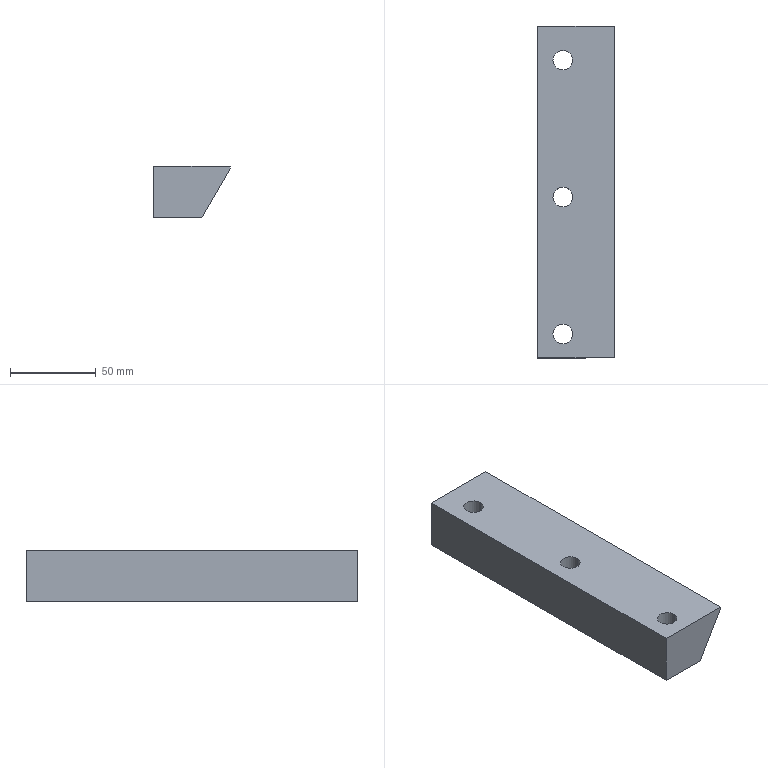Part | STEP file | NGAM TRUOT_3 | 1 solid | 13 faces | box 45 x 194 x 30 mm | volume 205453 mm3 | plane 7 | cylinder 6 | commonest cylinder face diameters 11.5 x6
STEP:
#1=CARTESIAN_POINT('',(0.,0.,0.));
#2=DIRECTION('',(0.,0.,1.));
#3=DIRECTION('',(1.,0.,0.));
#4=AXIS2_PLACEMENT_3D('',#1,#2,#3);
#5=CARTESIAN_POINT('',(20.55,180.,0.));
#6=VERTEX_POINT('',#5);
#7=CARTESIAN_POINT('',(20.55,180.,30.));
#8=VERTEX_POINT('',#7);
#9=CARTESIAN_POINT('',(20.55,180.,0.));
#10=DIRECTION('',(0.,0.,1.));
#11=VECTOR('',#10,1.);
#12=LINE('',#9,#11);
#13=CARTESIAN_POINT('',(14.8,180.,0.));
#14=DIRECTION('',(0.,0.,1.));
#15=DIRECTION('',(1.,0.,0.));
#16=AXIS2_PLACEMENT_3D('',#13,#14,#15);
#17=CYLINDRICAL_SURFACE('',#16,5.75);
#18=CARTESIAN_POINT('',(6.283,0.));
#19=DIRECTION('',(0.,1.));
#20=VECTOR('',#19,1.);
#21=LINE('',#18,#20);
#22=(GEOMETRIC_REPRESENTATION_CONTEXT(2)PARAMETRIC_REPRESENTATION_CONTEXT()REPRESENTATION_CONTEXT('',''));
#23=DEFINITIONAL_REPRESENTATION('',(#21),#22);
#24=PCURVE('',#17,#23);
#25=CARTESIAN_POINT('',(14.8,180.,0.));
#26=DIRECTION('',(0.,0.,1.));
#27=DIRECTION('',(1.,0.,0.));
#28=AXIS2_PLACEMENT_3D('',#25,#26,#27);
#29=CYLINDRICAL_SURFACE('',#28,5.75);
#30=CARTESIAN_POINT('',(0.,0.));
#31=DIRECTION('',(0.,1.));
#32=VECTOR('',#31,1.);
#33=LINE('',#30,#32);
#34=(GEOMETRIC_REPRESENTATION_CONTEXT(2)PARAMETRIC_REPRESENTATION_CONTEXT()REPRESENTATION_CONTEXT('',''));
#35=DEFINITIONAL_REPRESENTATION('',(#33),#34);
#36=PCURVE('',#29,#35);
#37=SURFACE_CURVE('',#12,(#24,#36),.PCURVE_S1.);
#38=EDGE_CURVE('',#6,#8,#37,.T.);
#39=ORIENTED_EDGE('',*,*,#38,.T.);
#40=CARTESIAN_POINT('',(9.05,180.,30.));
#41=VERTEX_POINT('',#40);
#42=CARTESIAN_POINT('',(14.8,180.,30.));
#43=DIRECTION('',(0.,0.,-1.));
#44=DIRECTION('',(1.,0.,0.));
#45=AXIS2_PLACEMENT_3D('',#42,#43,#44);
#46=CIRCLE('',#45,5.75);
#47=CARTESIAN_POINT('',(6.283,30.));
#48=DIRECTION('',(-1.,0.));
#49=VECTOR('',#48,1.);
#50=LINE('',#47,#49);
#51=(GEOMETRIC_REPRESENTATION_CONTEXT(2)PARAMETRIC_REPRESENTATION_CONTEXT()REPRESENTATION_CONTEXT('',''));
#52=DEFINITIONAL_REPRESENTATION('',(#50),#51);
#53=PCURVE('',#17,#52);
#54=CARTESIAN_POINT('',(22.5,100.,30.));
#55=DIRECTION('',(0.,0.,1.));
#56=DIRECTION('',(1.,0.,0.));
#57=AXIS2_PLACEMENT_3D('',#54,#55,#56);
#58=PLANE('',#57);
#59=CARTESIAN_POINT('',(-1.95,80.));
#60=CARTESIAN_POINT('',(-1.95,70.041));
#61=CARTESIAN_POINT('',(-10.575,75.02));
#62=CARTESIAN_POINT('',(-19.2,80.));
#63=CARTESIAN_POINT('',(-10.575,84.98));
#64=CARTESIAN_POINT('',(-1.95,89.959));
#65=CARTESIAN_POINT('',(-1.95,80.));
#66=(BOUNDED_CURVE()B_SPLINE_CURVE(2,(#59,#60,#61,#62,#63,#64,#65),.UNSPECIFIED.,.T.,.F.)B_SPLINE_CURVE_WITH_KNOTS((1,2,2,2,2,1),(-2.094,0.,2.094,4.189,6.283,8.378),.UNSPECIFIED.)CURVE()GEOMETRIC_REPRESENTATION_ITEM()RATIONAL_B_SPLINE_CURVE((1.,0.5,1.,0.5,1.,0.5,1.))REPRESENTATION_ITEM(''));
#67=(GEOMETRIC_REPRESENTATION_CONTEXT(2)PARAMETRIC_REPRESENTATION_CONTEXT()REPRESENTATION_CONTEXT('',''));
#68=DEFINITIONAL_REPRESENTATION('',(#66),#67);
#69=PCURVE('',#58,#68);
#70=SURFACE_CURVE('',#46,(#53,#69),.PCURVE_S1.);
#71=EDGE_CURVE('',#8,#41,#70,.T.);
#72=ORIENTED_EDGE('',*,*,#71,.T.);
#73=CARTESIAN_POINT('',(9.05,180.,0.));
#74=VERTEX_POINT('',#73);
#75=CARTESIAN_POINT('',(9.05,180.,0.));
#76=DIRECTION('',(0.,0.,1.));
#77=VECTOR('',#76,1.);
#78=LINE('',#75,#77);
#79=CARTESIAN_POINT('',(3.142,0.));
#80=DIRECTION('',(0.,1.));
#81=VECTOR('',#80,1.);
#82=LINE('',#79,#81);
#83=(GEOMETRIC_REPRESENTATION_CONTEXT(2)PARAMETRIC_REPRESENTATION_CONTEXT()REPRESENTATION_CONTEXT('',''));
#84=DEFINITIONAL_REPRESENTATION('',(#82),#83);
#85=PCURVE('',#17,#84);
#86=CARTESIAN_POINT('',(3.142,0.));
#87=DIRECTION('',(0.,1.));
#88=VECTOR('',#87,1.);
#89=LINE('',#86,#88);
#90=(GEOMETRIC_REPRESENTATION_CONTEXT(2)PARAMETRIC_REPRESENTATION_CONTEXT()REPRESENTATION_CONTEXT('',''));
#91=DEFINITIONAL_REPRESENTATION('',(#89),#90);
#92=PCURVE('',#29,#91);
#93=SURFACE_CURVE('',#78,(#85,#92),.PCURVE_S1.);
#94=EDGE_CURVE('',#74,#41,#93,.T.);
#95=ORIENTED_EDGE('',*,*,#94,.F.);
#96=CARTESIAN_POINT('',(14.8,180.,0.));
#97=DIRECTION('',(0.,0.,1.));
#98=DIRECTION('',(1.,0.,0.));
#99=AXIS2_PLACEMENT_3D('',#96,#97,#98);
#100=CIRCLE('',#99,5.75);
#101=CARTESIAN_POINT('',(0.,0.));
#102=DIRECTION('',(1.,0.));
#103=VECTOR('',#102,1.);
#104=LINE('',#101,#103);
#105=(GEOMETRIC_REPRESENTATION_CONTEXT(2)PARAMETRIC_REPRESENTATION_CONTEXT()REPRESENTATION_CONTEXT('',''));
#106=DEFINITIONAL_REPRESENTATION('',(#104),#105);
#107=PCURVE('',#17,#106);
#108=CARTESIAN_POINT('',(22.5,100.,0.));
#109=DIRECTION('',(0.,0.,1.));
#110=DIRECTION('',(1.,0.,0.));
#111=AXIS2_PLACEMENT_3D('',#108,#109,#110);
#112=PLANE('',#111);
#113=CARTESIAN_POINT('',(-7.7,80.));
#114=DIRECTION('',(1.,0.));
#115=AXIS2_PLACEMENT_2D('',#113,#114);
#116=CIRCLE('',#115,5.75);
#117=(GEOMETRIC_REPRESENTATION_CONTEXT(2)PARAMETRIC_REPRESENTATION_CONTEXT()REPRESENTATION_CONTEXT('',''));
#118=DEFINITIONAL_REPRESENTATION('',(#116),#117);
#119=PCURVE('',#112,#118);
#120=SURFACE_CURVE('',#100,(#107,#119),.PCURVE_S1.);
#121=EDGE_CURVE('',#74,#6,#120,.T.);
#122=ORIENTED_EDGE('',*,*,#121,.T.);
#123=EDGE_LOOP('',(#39,#72,#95,#122));
#124=FACE_BOUND('',#123,.F.);
#125=ADVANCED_FACE('',(#124),#17,.F.);
#126=CARTESIAN_POINT('',(20.55,100.,0.));
#127=VERTEX_POINT('',#126);
#128=CARTESIAN_POINT('',(20.55,100.,30.));
#129=VERTEX_POINT('',#128);
#130=CARTESIAN_POINT('',(20.55,100.,0.));
#131=DIRECTION('',(0.,0.,1.));
#132=VECTOR('',#131,1.);
#133=LINE('',#130,#132);
#134=CARTESIAN_POINT('',(14.8,100.,0.));
#135=DIRECTION('',(0.,0.,1.));
#136=DIRECTION('',(1.,0.,0.));
#137=AXIS2_PLACEMENT_3D('',#134,#135,#136);
#138=CYLINDRICAL_SURFACE('',#137,5.75);
#139=CARTESIAN_POINT('',(6.283,0.));
#140=DIRECTION('',(0.,1.));
#141=VECTOR('',#140,1.);
#142=LINE('',#139,#141);
#143=(GEOMETRIC_REPRESENTATION_CONTEXT(2)PARAMETRIC_REPRESENTATION_CONTEXT()REPRESENTATION_CONTEXT('',''));
#144=DEFINITIONAL_REPRESENTATION('',(#142),#143);
#145=PCURVE('',#138,#144);
#146=CARTESIAN_POINT('',(14.8,100.,0.));
#147=DIRECTION('',(0.,0.,1.));
#148=DIRECTION('',(1.,0.,0.));
#149=AXIS2_PLACEMENT_3D('',#146,#147,#148);
#150=CYLINDRICAL_SURFACE('',#149,5.75);
#151=CARTESIAN_POINT('',(0.,0.));
#152=DIRECTION('',(0.,1.));
#153=VECTOR('',#152,1.);
#154=LINE('',#151,#153);
#155=(GEOMETRIC_REPRESENTATION_CONTEXT(2)PARAMETRIC_REPRESENTATION_CONTEXT()REPRESENTATION_CONTEXT('',''));
#156=DEFINITIONAL_REPRESENTATION('',(#154),#155);
#157=PCURVE('',#150,#156);
#158=SURFACE_CURVE('',#133,(#145,#157),.PCURVE_S1.);
#159=EDGE_CURVE('',#127,#129,#158,.T.);
#160=ORIENTED_EDGE('',*,*,#159,.T.);
#161=CARTESIAN_POINT('',(9.05,100.,30.));
#162=VERTEX_POINT('',#161);
#163=CARTESIAN_POINT('',(14.8,100.,30.));
#164=DIRECTION('',(0.,0.,-1.));
#165=DIRECTION('',(1.,0.,0.));
#166=AXIS2_PLACEMENT_3D('',#163,#164,#165);
#167=CIRCLE('',#166,5.75);
#168=CARTESIAN_POINT('',(6.283,30.));
#169=DIRECTION('',(-1.,0.));
#170=VECTOR('',#169,1.);
#171=LINE('',#168,#170);
#172=(GEOMETRIC_REPRESENTATION_CONTEXT(2)PARAMETRIC_REPRESENTATION_CONTEXT()REPRESENTATION_CONTEXT('',''));
#173=DEFINITIONAL_REPRESENTATION('',(#171),#172);
#174=PCURVE('',#138,#173);
#175=CARTESIAN_POINT('',(-1.95,0.));
#176=CARTESIAN_POINT('',(-1.95,-9.959));
#177=CARTESIAN_POINT('',(-10.575,-4.98));
#178=CARTESIAN_POINT('',(-19.2,0.));
#179=CARTESIAN_POINT('',(-10.575,4.98));
#180=CARTESIAN_POINT('',(-1.95,9.959));
#181=CARTESIAN_POINT('',(-1.95,0.));
#182=(BOUNDED_CURVE()B_SPLINE_CURVE(2,(#175,#176,#177,#178,#179,#180,#181),.UNSPECIFIED.,.T.,.F.)B_SPLINE_CURVE_WITH_KNOTS((1,2,2,2,2,1),(-2.094,0.,2.094,4.189,6.283,8.378),.UNSPECIFIED.)CURVE()GEOMETRIC_REPRESENTATION_ITEM()RATIONAL_B_SPLINE_CURVE((1.,0.5,1.,0.5,1.,0.5,1.))REPRESENTATION_ITEM(''));
#183=(GEOMETRIC_REPRESENTATION_CONTEXT(2)PARAMETRIC_REPRESENTATION_CONTEXT()REPRESENTATION_CONTEXT('',''));
#184=DEFINITIONAL_REPRESENTATION('',(#182),#183);
#185=PCURVE('',#58,#184);
#186=SURFACE_CURVE('',#167,(#174,#185),.PCURVE_S1.);
#187=EDGE_CURVE('',#129,#162,#186,.T.);
#188=ORIENTED_EDGE('',*,*,#187,.T.);
#189=CARTESIAN_POINT('',(9.05,100.,0.));
#190=VERTEX_POINT('',#189);
#191=CARTESIAN_POINT('',(9.05,100.,0.));
#192=DIRECTION('',(0.,0.,1.));
#193=VECTOR('',#192,1.);
#194=LINE('',#191,#193);
#195=CARTESIAN_POINT('',(3.142,0.));
#196=DIRECTION('',(0.,1.));
#197=VECTOR('',#196,1.);
#198=LINE('',#195,#197);
#199=(GEOMETRIC_REPRESENTATION_CONTEXT(2)PARAMETRIC_REPRESENTATION_CONTEXT()REPRESENTATION_CONTEXT('',''));
#200=DEFINITIONAL_REPRESENTATION('',(#198),#199);
#201=PCURVE('',#138,#200);
#202=CARTESIAN_POINT('',(3.142,0.));
#203=DIRECTION('',(0.,1.));
#204=VECTOR('',#203,1.);
#205=LINE('',#202,#204);
#206=(GEOMETRIC_REPRESENTATION_CONTEXT(2)PARAMETRIC_REPRESENTATION_CONTEXT()REPRESENTATION_CONTEXT('',''));
#207=DEFINITIONAL_REPRESENTATION('',(#205),#206);
#208=PCURVE('',#150,#207);
#209=SURFACE_CURVE('',#194,(#201,#208),.PCURVE_S1.);
#210=EDGE_CURVE('',#190,#162,#209,.T.);
#211=ORIENTED_EDGE('',*,*,#210,.F.);
#212=CARTESIAN_POINT('',(14.8,100.,0.));
#213=DIRECTION('',(0.,0.,1.));
#214=DIRECTION('',(1.,0.,0.));
#215=AXIS2_PLACEMENT_3D('',#212,#213,#214);
#216=CIRCLE('',#215,5.75);
#217=CARTESIAN_POINT('',(0.,0.));
#218=DIRECTION('',(1.,0.));
#219=VECTOR('',#218,1.);
#220=LINE('',#217,#219);
#221=(GEOMETRIC_REPRESENTATION_CONTEXT(2)PARAMETRIC_REPRESENTATION_CONTEXT()REPRESENTATION_CONTEXT('',''));
#222=DEFINITIONAL_REPRESENTATION('',(#220),#221);
#223=PCURVE('',#138,#222);
#224=CARTESIAN_POINT('',(-7.7,0.));
#225=DIRECTION('',(1.,0.));
#226=AXIS2_PLACEMENT_2D('',#224,#225);
#227=CIRCLE('',#226,5.75);
#228=(GEOMETRIC_REPRESENTATION_CONTEXT(2)PARAMETRIC_REPRESENTATION_CONTEXT()REPRESENTATION_CONTEXT('',''));
#229=DEFINITIONAL_REPRESENTATION('',(#227),#228);
#230=PCURVE('',#112,#229);
#231=SURFACE_CURVE('',#216,(#223,#230),.PCURVE_S1.);
#232=EDGE_CURVE('',#190,#127,#231,.T.);
#233=ORIENTED_EDGE('',*,*,#232,.T.);
#234=EDGE_LOOP('',(#160,#188,#211,#233));
#235=FACE_BOUND('',#234,.F.);
#236=ADVANCED_FACE('',(#235),#138,.F.);
#237=CARTESIAN_POINT('',(20.55,20.,0.));
#238=VERTEX_POINT('',#237);
#239=CARTESIAN_POINT('',(20.55,20.,30.));
#240=VERTEX_POINT('',#239);
#241=CARTESIAN_POINT('',(20.55,20.,0.));
#242=DIRECTION('',(0.,0.,1.));
#243=VECTOR('',#242,1.);
#244=LINE('',#241,#243);
#245=CARTESIAN_POINT('',(14.8,20.,0.));
#246=DIRECTION('',(0.,0.,1.));
#247=DIRECTION('',(1.,0.,0.));
#248=AXIS2_PLACEMENT_3D('',#245,#246,#247);
#249=CYLINDRICAL_SURFACE('',#248,5.75);
#250=CARTESIAN_POINT('',(6.283,0.));
#251=DIRECTION('',(0.,1.));
#252=VECTOR('',#251,1.);
#253=LINE('',#250,#252);
#254=(GEOMETRIC_REPRESENTATION_CONTEXT(2)PARAMETRIC_REPRESENTATION_CONTEXT()REPRESENTATION_CONTEXT('',''));
#255=DEFINITIONAL_REPRESENTATION('',(#253),#254);
#256=PCURVE('',#249,#255);
#257=CARTESIAN_POINT('',(14.8,20.,0.));
#258=DIRECTION('',(0.,0.,1.));
#259=DIRECTION('',(1.,0.,0.));
#260=AXIS2_PLACEMENT_3D('',#257,#258,#259);
#261=CYLINDRICAL_SURFACE('',#260,5.75);
#262=CARTESIAN_POINT('',(0.,0.));
#263=DIRECTION('',(0.,1.));
#264=VECTOR('',#263,1.);
#265=LINE('',#262,#264);
#266=(GEOMETRIC_REPRESENTATION_CONTEXT(2)PARAMETRIC_REPRESENTATION_CONTEXT()REPRESENTATION_CONTEXT('',''));
#267=DEFINITIONAL_REPRESENTATION('',(#265),#266);
#268=PCURVE('',#261,#267);
#269=SURFACE_CURVE('',#244,(#256,#268),.PCURVE_S1.);
#270=EDGE_CURVE('',#238,#240,#269,.T.);
#271=ORIENTED_EDGE('',*,*,#270,.T.);
#272=CARTESIAN_POINT('',(9.05,20.,30.));
#273=VERTEX_POINT('',#272);
#274=CARTESIAN_POINT('',(14.8,20.,30.));
#275=DIRECTION('',(0.,0.,-1.));
#276=DIRECTION('',(1.,0.,0.));
#277=AXIS2_PLACEMENT_3D('',#274,#275,#276);
#278=CIRCLE('',#277,5.75);
#279=CARTESIAN_POINT('',(6.283,30.));
#280=DIRECTION('',(-1.,0.));
#281=VECTOR('',#280,1.);
#282=LINE('',#279,#281);
#283=(GEOMETRIC_REPRESENTATION_CONTEXT(2)PARAMETRIC_REPRESENTATION_CONTEXT()REPRESENTATION_CONTEXT('',''));
#284=DEFINITIONAL_REPRESENTATION('',(#282),#283);
#285=PCURVE('',#249,#284);
#286=CARTESIAN_POINT('',(-1.95,-80.));
#287=CARTESIAN_POINT('',(-1.95,-89.959));
#288=CARTESIAN_POINT('',(-10.575,-84.98));
#289=CARTESIAN_POINT('',(-19.2,-80.));
#290=CARTESIAN_POINT('',(-10.575,-75.02));
#291=CARTESIAN_POINT('',(-1.95,-70.041));
#292=CARTESIAN_POINT('',(-1.95,-80.));
#293=(BOUNDED_CURVE()B_SPLINE_CURVE(2,(#286,#287,#288,#289,#290,#291,#292),.UNSPECIFIED.,.T.,.F.)B_SPLINE_CURVE_WITH_KNOTS((1,2,2,2,2,1),(-2.094,0.,2.094,4.189,6.283,8.378),.UNSPECIFIED.)CURVE()GEOMETRIC_REPRESENTATION_ITEM()RATIONAL_B_SPLINE_CURVE((1.,0.5,1.,0.5,1.,0.5,1.))REPRESENTATION_ITEM(''));
#294=(GEOMETRIC_REPRESENTATION_CONTEXT(2)PARAMETRIC_REPRESENTATION_CONTEXT()REPRESENTATION_CONTEXT('',''));
#295=DEFINITIONAL_REPRESENTATION('',(#293),#294);
#296=PCURVE('',#58,#295);
#297=SURFACE_CURVE('',#278,(#285,#296),.PCURVE_S1.);
#298=EDGE_CURVE('',#240,#273,#297,.T.);
#299=ORIENTED_EDGE('',*,*,#298,.T.);
#300=CARTESIAN_POINT('',(9.05,20.,0.));
#301=VERTEX_POINT('',#300);
#302=CARTESIAN_POINT('',(9.05,20.,0.));
#303=DIRECTION('',(0.,0.,1.));
#304=VECTOR('',#303,1.);
#305=LINE('',#302,#304);
#306=CARTESIAN_POINT('',(3.142,0.));
#307=DIRECTION('',(0.,1.));
#308=VECTOR('',#307,1.);
#309=LINE('',#306,#308);
#310=(GEOMETRIC_REPRESENTATION_CONTEXT(2)PARAMETRIC_REPRESENTATION_CONTEXT()REPRESENTATION_CONTEXT('',''));
#311=DEFINITIONAL_REPRESENTATION('',(#309),#310);
#312=PCURVE('',#249,#311);
#313=CARTESIAN_POINT('',(3.142,0.));
#314=DIRECTION('',(0.,1.));
#315=VECTOR('',#314,1.);
#316=LINE('',#313,#315);
#317=(GEOMETRIC_REPRESENTATION_CONTEXT(2)PARAMETRIC_REPRESENTATION_CONTEXT()REPRESENTATION_CONTEXT('',''));
#318=DEFINITIONAL_REPRESENTATION('',(#316),#317);
#319=PCURVE('',#261,#318);
#320=SURFACE_CURVE('',#305,(#312,#319),.PCURVE_S1.);
#321=EDGE_CURVE('',#301,#273,#320,.T.);
#322=ORIENTED_EDGE('',*,*,#321,.F.);
#323=CARTESIAN_POINT('',(14.8,20.,0.));
#324=DIRECTION('',(0.,0.,1.));
#325=DIRECTION('',(1.,0.,0.));
#326=AXIS2_PLACEMENT_3D('',#323,#324,#325);
#327=CIRCLE('',#326,5.75);
#328=CARTESIAN_POINT('',(0.,0.));
#329=DIRECTION('',(1.,0.));
#330=VECTOR('',#329,1.);
#331=LINE('',#328,#330);
#332=(GEOMETRIC_REPRESENTATION_CONTEXT(2)PARAMETRIC_REPRESENTATION_CONTEXT()REPRESENTATION_CONTEXT('',''));
#333=DEFINITIONAL_REPRESENTATION('',(#331),#332);
#334=PCURVE('',#249,#333);
#335=CARTESIAN_POINT('',(-7.7,-80.));
#336=DIRECTION('',(1.,0.));
#337=AXIS2_PLACEMENT_2D('',#335,#336);
#338=CIRCLE('',#337,5.75);
#339=(GEOMETRIC_REPRESENTATION_CONTEXT(2)PARAMETRIC_REPRESENTATION_CONTEXT()REPRESENTATION_CONTEXT('',''));
#340=DEFINITIONAL_REPRESENTATION('',(#338),#339);
#341=PCURVE('',#112,#340);
#342=SURFACE_CURVE('',#327,(#334,#341),.PCURVE_S1.);
#343=EDGE_CURVE('',#301,#238,#342,.T.);
#344=ORIENTED_EDGE('',*,*,#343,.T.);
#345=EDGE_LOOP('',(#271,#299,#322,#344));
#346=FACE_BOUND('',#345,.F.);
#347=ADVANCED_FACE('',(#346),#249,.F.);
#348=ORIENTED_EDGE('',*,*,#71,.T.);
#349=CARTESIAN_POINT('',(14.8,180.,30.));
#350=DIRECTION('',(0.,0.,-1.));
#351=DIRECTION('',(1.,0.,0.));
#352=AXIS2_PLACEMENT_3D('',#349,#350,#351);
#353=CIRCLE('',#352,5.75);
#354=CARTESIAN_POINT('',(-1.95,80.));
#355=CARTESIAN_POINT('',(-1.95,70.041));
#356=CARTESIAN_POINT('',(-10.575,75.02));
#357=CARTESIAN_POINT('',(-19.2,80.));
#358=CARTESIAN_POINT('',(-10.575,84.98));
#359=CARTESIAN_POINT('',(-1.95,89.959));
#360=CARTESIAN_POINT('',(-1.95,80.));
#361=(BOUNDED_CURVE()B_SPLINE_CURVE(2,(#354,#355,#356,#357,#358,#359,#360),.UNSPECIFIED.,.T.,.F.)B_SPLINE_CURVE_WITH_KNOTS((1,2,2,2,2,1),(-2.094,0.,2.094,4.189,6.283,8.378),.UNSPECIFIED.)CURVE()GEOMETRIC_REPRESENTATION_ITEM()RATIONAL_B_SPLINE_CURVE((1.,0.5,1.,0.5,1.,0.5,1.))REPRESENTATION_ITEM(''));
#362=(GEOMETRIC_REPRESENTATION_CONTEXT(2)PARAMETRIC_REPRESENTATION_CONTEXT()REPRESENTATION_CONTEXT('',''));
#363=DEFINITIONAL_REPRESENTATION('',(#361),#362);
#364=PCURVE('',#58,#363);
#365=CARTESIAN_POINT('',(6.283,30.));
#366=DIRECTION('',(-1.,0.));
#367=VECTOR('',#366,1.);
#368=LINE('',#365,#367);
#369=(GEOMETRIC_REPRESENTATION_CONTEXT(2)PARAMETRIC_REPRESENTATION_CONTEXT()REPRESENTATION_CONTEXT('',''));
#370=DEFINITIONAL_REPRESENTATION('',(#368),#369);
#371=PCURVE('',#29,#370);
#372=SURFACE_CURVE('',#353,(#364,#371),.PCURVE_S1.);
#373=EDGE_CURVE('',#41,#8,#372,.T.);
#374=ORIENTED_EDGE('',*,*,#373,.T.);
#375=EDGE_LOOP('',(#348,#374));
#376=FACE_BOUND('',#375,.T.);
#377=ORIENTED_EDGE('',*,*,#187,.T.);
#378=CARTESIAN_POINT('',(14.8,100.,30.));
#379=DIRECTION('',(0.,0.,-1.));
#380=DIRECTION('',(1.,0.,0.));
#381=AXIS2_PLACEMENT_3D('',#378,#379,#380);
#382=CIRCLE('',#381,5.75);
#383=CARTESIAN_POINT('',(-1.95,0.));
#384=CARTESIAN_POINT('',(-1.95,-9.959));
#385=CARTESIAN_POINT('',(-10.575,-4.98));
#386=CARTESIAN_POINT('',(-19.2,0.));
#387=CARTESIAN_POINT('',(-10.575,4.98));
#388=CARTESIAN_POINT('',(-1.95,9.959));
#389=CARTESIAN_POINT('',(-1.95,0.));
#390=(BOUNDED_CURVE()B_SPLINE_CURVE(2,(#383,#384,#385,#386,#387,#388,#389),.UNSPECIFIED.,.T.,.F.)B_SPLINE_CURVE_WITH_KNOTS((1,2,2,2,2,1),(-2.094,0.,2.094,4.189,6.283,8.378),.UNSPECIFIED.)CURVE()GEOMETRIC_REPRESENTATION_ITEM()RATIONAL_B_SPLINE_CURVE((1.,0.5,1.,0.5,1.,0.5,1.))REPRESENTATION_ITEM(''));
#391=(GEOMETRIC_REPRESENTATION_CONTEXT(2)PARAMETRIC_REPRESENTATION_CONTEXT()REPRESENTATION_CONTEXT('',''));
#392=DEFINITIONAL_REPRESENTATION('',(#390),#391);
#393=PCURVE('',#58,#392);
#394=CARTESIAN_POINT('',(6.283,30.));
#395=DIRECTION('',(-1.,0.));
#396=VECTOR('',#395,1.);
#397=LINE('',#394,#396);
#398=(GEOMETRIC_REPRESENTATION_CONTEXT(2)PARAMETRIC_REPRESENTATION_CONTEXT()REPRESENTATION_CONTEXT('',''));
#399=DEFINITIONAL_REPRESENTATION('',(#397),#398);
#400=PCURVE('',#150,#399);
#401=SURFACE_CURVE('',#382,(#393,#400),.PCURVE_S1.);
#402=EDGE_CURVE('',#162,#129,#401,.T.);
#403=ORIENTED_EDGE('',*,*,#402,.T.);
#404=EDGE_LOOP('',(#377,#403));
#405=FACE_BOUND('',#404,.T.);
#406=ORIENTED_EDGE('',*,*,#298,.T.);
#407=CARTESIAN_POINT('',(14.8,20.,30.));
#408=DIRECTION('',(0.,0.,-1.));
#409=DIRECTION('',(1.,0.,0.));
#410=AXIS2_PLACEMENT_3D('',#407,#408,#409);
#411=CIRCLE('',#410,5.75);
#412=CARTESIAN_POINT('',(-1.95,-80.));
#413=CARTESIAN_POINT('',(-1.95,-89.959));
#414=CARTESIAN_POINT('',(-10.575,-84.98));
#415=CARTESIAN_POINT('',(-19.2,-80.));
#416=CARTESIAN_POINT('',(-10.575,-75.02));
#417=CARTESIAN_POINT('',(-1.95,-70.041));
#418=CARTESIAN_POINT('',(-1.95,-80.));
#419=(BOUNDED_CURVE()B_SPLINE_CURVE(2,(#412,#413,#414,#415,#416,#417,#418),.UNSPECIFIED.,.T.,.F.)B_SPLINE_CURVE_WITH_KNOTS((1,2,2,2,2,1),(-2.094,0.,2.094,4.189,6.283,8.378),.UNSPECIFIED.)CURVE()GEOMETRIC_REPRESENTATION_ITEM()RATIONAL_B_SPLINE_CURVE((1.,0.5,1.,0.5,1.,0.5,1.))REPRESENTATION_ITEM(''));
#420=(GEOMETRIC_REPRESENTATION_CONTEXT(2)PARAMETRIC_REPRESENTATION_CONTEXT()REPRESENTATION_CONTEXT('',''));
#421=DEFINITIONAL_REPRESENTATION('',(#419),#420);
#422=PCURVE('',#58,#421);
#423=CARTESIAN_POINT('',(6.283,30.));
#424=DIRECTION('',(-1.,0.));
#425=VECTOR('',#424,1.);
#426=LINE('',#423,#425);
#427=(GEOMETRIC_REPRESENTATION_CONTEXT(2)PARAMETRIC_REPRESENTATION_CONTEXT()REPRESENTATION_CONTEXT('',''));
#428=DEFINITIONAL_REPRESENTATION('',(#426),#427);
#429=PCURVE('',#261,#428);
#430=SURFACE_CURVE('',#411,(#422,#429),.PCURVE_S1.);
#431=EDGE_CURVE('',#273,#240,#430,.T.);
#432=ORIENTED_EDGE('',*,*,#431,.T.);
#433=EDGE_LOOP('',(#406,#432));
#434=FACE_BOUND('',#433,.T.);
#435=CARTESIAN_POINT('',(45.,200.,30.));
#436=VERTEX_POINT('',#435);
#437=CARTESIAN_POINT('',(0.,200.,30.));
#438=VERTEX_POINT('',#437);
#439=CARTESIAN_POINT('',(22.5,200.,30.));
#440=DIRECTION('',(-1.,0.,0.));
#441=VECTOR('',#440,1.);
#442=LINE('',#439,#441);
#443=CARTESIAN_POINT('',(0.,100.));
#444=DIRECTION('',(-1.,0.));
#445=VECTOR('',#444,1.);
#446=LINE('',#443,#445);
#447=(GEOMETRIC_REPRESENTATION_CONTEXT(2)PARAMETRIC_REPRESENTATION_CONTEXT()REPRESENTATION_CONTEXT('',''));
#448=DEFINITIONAL_REPRESENTATION('',(#446),#447);
#449=PCURVE('',#58,#448);
#450=CARTESIAN_POINT('',(0.,200.,0.));
#451=DIRECTION('',(0.,1.,0.));
#452=DIRECTION('',(0.,0.,1.));
#453=AXIS2_PLACEMENT_3D('',#450,#451,#452);
#454=PLANE('',#453);
#455=CARTESIAN_POINT('',(30.,22.5));
#456=DIRECTION('',(0.,-1.));
#457=VECTOR('',#456,1.);
#458=LINE('',#455,#457);
#459=(GEOMETRIC_REPRESENTATION_CONTEXT(2)PARAMETRIC_REPRESENTATION_CONTEXT()REPRESENTATION_CONTEXT('',''));
#460=DEFINITIONAL_REPRESENTATION('',(#458),#459);
#461=PCURVE('',#454,#460);
#462=SURFACE_CURVE('',#442,(#449,#461),.PCURVE_S1.);
#463=EDGE_CURVE('',#436,#438,#462,.T.);
#464=ORIENTED_EDGE('',*,*,#463,.T.);
#465=CARTESIAN_POINT('',(0.,6.,30.));
#466=VERTEX_POINT('',#465);
#467=CARTESIAN_POINT('',(0.,100.,30.));
#468=DIRECTION('',(0.,-1.,0.));
#469=VECTOR('',#468,1.);
#470=LINE('',#467,#469);
#471=CARTESIAN_POINT('',(-22.5,0.));
#472=DIRECTION('',(0.,-1.));
#473=VECTOR('',#472,1.);
#474=LINE('',#471,#473);
#475=(GEOMETRIC_REPRESENTATION_CONTEXT(2)PARAMETRIC_REPRESENTATION_CONTEXT()REPRESENTATION_CONTEXT('',''));
#476=DEFINITIONAL_REPRESENTATION('',(#474),#475);
#477=PCURVE('',#58,#476);
#478=CARTESIAN_POINT('',(0.,0.,0.));
#479=DIRECTION('',(-1.,0.,0.));
#480=DIRECTION('',(0.,0.,1.));
#481=AXIS2_PLACEMENT_3D('',#478,#479,#480);
#482=PLANE('',#481);
#483=CARTESIAN_POINT('',(30.,100.));
#484=DIRECTION('',(0.,-1.));
#485=VECTOR('',#484,1.);
#486=LINE('',#483,#485);
#487=(GEOMETRIC_REPRESENTATION_CONTEXT(2)PARAMETRIC_REPRESENTATION_CONTEXT()REPRESENTATION_CONTEXT('',''));
#488=DEFINITIONAL_REPRESENTATION('',(#486),#487);
#489=PCURVE('',#482,#488);
#490=SURFACE_CURVE('',#470,(#477,#489),.PCURVE_S1.);
#491=EDGE_CURVE('',#438,#466,#490,.T.);
#492=ORIENTED_EDGE('',*,*,#491,.T.);
#493=CARTESIAN_POINT('',(45.,6.,30.));
#494=VERTEX_POINT('',#493);
#495=CARTESIAN_POINT('',(22.5,6.,30.));
#496=DIRECTION('',(1.,0.,0.));
#497=VECTOR('',#496,1.);
#498=LINE('',#495,#497);
#499=CARTESIAN_POINT('',(0.,-94.));
#500=DIRECTION('',(1.,0.));
#501=VECTOR('',#500,1.);
#502=LINE('',#499,#501);
#503=(GEOMETRIC_REPRESENTATION_CONTEXT(2)PARAMETRIC_REPRESENTATION_CONTEXT()REPRESENTATION_CONTEXT('',''));
#504=DEFINITIONAL_REPRESENTATION('',(#502),#503);
#505=PCURVE('',#58,#504);
#506=CARTESIAN_POINT('',(19.48,6.,16.807));
#507=DIRECTION('',(0.,1.,0.));
#508=DIRECTION('',(0.,0.,1.));
#509=AXIS2_PLACEMENT_3D('',#506,#507,#508);
#510=PLANE('',#509);
#511=CARTESIAN_POINT('',(13.193,3.02));
#512=DIRECTION('',(0.,1.));
#513=VECTOR('',#512,1.);
#514=LINE('',#511,#513);
#515=(GEOMETRIC_REPRESENTATION_CONTEXT(2)PARAMETRIC_REPRESENTATION_CONTEXT()REPRESENTATION_CONTEXT('',''));
#516=DEFINITIONAL_REPRESENTATION('',(#514),#515);
#517=PCURVE('',#510,#516);
#518=SURFACE_CURVE('',#498,(#505,#517),.PCURVE_S1.);
#519=EDGE_CURVE('',#466,#494,#518,.T.);
#520=ORIENTED_EDGE('',*,*,#519,.T.);
#521=CARTESIAN_POINT('',(45.,100.,30.));
#522=DIRECTION('',(0.,1.,0.));
#523=VECTOR('',#522,1.);
#524=LINE('',#521,#523);
#525=CARTESIAN_POINT('',(22.5,0.));
#526=DIRECTION('',(0.,1.));
#527=VECTOR('',#526,1.);
#528=LINE('',#525,#527);
#529=(GEOMETRIC_REPRESENTATION_CONTEXT(2)PARAMETRIC_REPRESENTATION_CONTEXT()REPRESENTATION_CONTEXT('',''));
#530=DEFINITIONAL_REPRESENTATION('',(#528),#529);
#531=PCURVE('',#58,#530);
#532=CARTESIAN_POINT('',(45.,200.,0.));
#533=DIRECTION('',(1.,0.,0.));
#534=DIRECTION('',(0.,0.,-1.));
#535=AXIS2_PLACEMENT_3D('',#532,#533,#534);
#536=PLANE('',#535);
#537=CARTESIAN_POINT('',(-30.,-100.));
#538=DIRECTION('',(0.,1.));
#539=VECTOR('',#538,1.);
#540=LINE('',#537,#539);
#541=(GEOMETRIC_REPRESENTATION_CONTEXT(2)PARAMETRIC_REPRESENTATION_CONTEXT()REPRESENTATION_CONTEXT('',''));
#542=DEFINITIONAL_REPRESENTATION('',(#540),#541);
#543=PCURVE('',#536,#542);
#544=SURFACE_CURVE('',#524,(#531,#543),.PCURVE_S1.);
#545=EDGE_CURVE('',#494,#436,#544,.T.);
#546=ORIENTED_EDGE('',*,*,#545,.T.);
#547=EDGE_LOOP('',(#464,#492,#520,#546));
#548=FACE_BOUND('',#547,.T.);
#549=ADVANCED_FACE('',(#376,#405,#434,#548),#58,.T.);
#550=ORIENTED_EDGE('',*,*,#373,.T.);
#551=ORIENTED_EDGE('',*,*,#38,.F.);
#552=CARTESIAN_POINT('',(14.8,180.,0.));
#553=DIRECTION('',(0.,0.,1.));
#554=DIRECTION('',(1.,0.,0.));
#555=AXIS2_PLACEMENT_3D('',#552,#553,#554);
#556=CIRCLE('',#555,5.75);
#557=CARTESIAN_POINT('',(0.,0.));
#558=DIRECTION('',(1.,0.));
#559=VECTOR('',#558,1.);
#560=LINE('',#557,#559);
#561=(GEOMETRIC_REPRESENTATION_CONTEXT(2)PARAMETRIC_REPRESENTATION_CONTEXT()REPRESENTATION_CONTEXT('',''));
#562=DEFINITIONAL_REPRESENTATION('',(#560),#561);
#563=PCURVE('',#29,#562);
#564=CARTESIAN_POINT('',(-7.7,80.));
#565=DIRECTION('',(1.,0.));
#566=AXIS2_PLACEMENT_2D('',#564,#565);
#567=CIRCLE('',#566,5.75);
#568=(GEOMETRIC_REPRESENTATION_CONTEXT(2)PARAMETRIC_REPRESENTATION_CONTEXT()REPRESENTATION_CONTEXT('',''));
#569=DEFINITIONAL_REPRESENTATION('',(#567),#568);
#570=PCURVE('',#112,#569);
#571=SURFACE_CURVE('',#556,(#563,#570),.PCURVE_S1.);
#572=EDGE_CURVE('',#6,#74,#571,.T.);
#573=ORIENTED_EDGE('',*,*,#572,.T.);
#574=ORIENTED_EDGE('',*,*,#94,.T.);
#575=EDGE_LOOP('',(#550,#551,#573,#574));
#576=FACE_BOUND('',#575,.F.);
#577=ADVANCED_FACE('',(#576),#29,.F.);
#578=ORIENTED_EDGE('',*,*,#402,.T.);
#579=ORIENTED_EDGE('',*,*,#159,.F.);
#580=CARTESIAN_POINT('',(14.8,100.,0.));
#581=DIRECTION('',(0.,0.,1.));
#582=DIRECTION('',(1.,0.,0.));
#583=AXIS2_PLACEMENT_3D('',#580,#581,#582);
#584=CIRCLE('',#583,5.75);
#585=CARTESIAN_POINT('',(0.,0.));
#586=DIRECTION('',(1.,0.));
#587=VECTOR('',#586,1.);
#588=LINE('',#585,#587);
#589=(GEOMETRIC_REPRESENTATION_CONTEXT(2)PARAMETRIC_REPRESENTATION_CONTEXT()REPRESENTATION_CONTEXT('',''));
#590=DEFINITIONAL_REPRESENTATION('',(#588),#589);
#591=PCURVE('',#150,#590);
#592=CARTESIAN_POINT('',(-7.7,0.));
#593=DIRECTION('',(1.,0.));
#594=AXIS2_PLACEMENT_2D('',#592,#593);
#595=CIRCLE('',#594,5.75);
#596=(GEOMETRIC_REPRESENTATION_CONTEXT(2)PARAMETRIC_REPRESENTATION_CONTEXT()REPRESENTATION_CONTEXT('',''));
#597=DEFINITIONAL_REPRESENTATION('',(#595),#596);
#598=PCURVE('',#112,#597);
#599=SURFACE_CURVE('',#584,(#591,#598),.PCURVE_S1.);
#600=EDGE_CURVE('',#127,#190,#599,.T.);
#601=ORIENTED_EDGE('',*,*,#600,.T.);
#602=ORIENTED_EDGE('',*,*,#210,.T.);
#603=EDGE_LOOP('',(#578,#579,#601,#602));
#604=FACE_BOUND('',#603,.F.);
#605=ADVANCED_FACE('',(#604),#150,.F.);
#606=ORIENTED_EDGE('',*,*,#431,.T.);
#607=ORIENTED_EDGE('',*,*,#270,.F.);
#608=CARTESIAN_POINT('',(14.8,20.,0.));
#609=DIRECTION('',(0.,0.,1.));
#610=DIRECTION('',(1.,0.,0.));
#611=AXIS2_PLACEMENT_3D('',#608,#609,#610);
#612=CIRCLE('',#611,5.75);
#613=CARTESIAN_POINT('',(0.,0.));
#614=DIRECTION('',(1.,0.));
#615=VECTOR('',#614,1.);
#616=LINE('',#613,#615);
#617=(GEOMETRIC_REPRESENTATION_CONTEXT(2)PARAMETRIC_REPRESENTATION_CONTEXT()REPRESENTATION_CONTEXT('',''));
#618=DEFINITIONAL_REPRESENTATION('',(#616),#617);
#619=PCURVE('',#261,#618);
#620=CARTESIAN_POINT('',(-7.7,-80.));
#621=DIRECTION('',(1.,0.));
#622=AXIS2_PLACEMENT_2D('',#620,#621);
#623=CIRCLE('',#622,5.75);
#624=(GEOMETRIC_REPRESENTATION_CONTEXT(2)PARAMETRIC_REPRESENTATION_CONTEXT()REPRESENTATION_CONTEXT('',''));
#625=DEFINITIONAL_REPRESENTATION('',(#623),#624);
#626=PCURVE('',#112,#625);
#627=SURFACE_CURVE('',#612,(#619,#626),.PCURVE_S1.);
#628=EDGE_CURVE('',#238,#301,#627,.T.);
#629=ORIENTED_EDGE('',*,*,#628,.T.);
#630=ORIENTED_EDGE('',*,*,#321,.T.);
#631=EDGE_LOOP('',(#606,#607,#629,#630));
#632=FACE_BOUND('',#631,.F.);
#633=ADVANCED_FACE('',(#632),#261,.F.);
#634=CARTESIAN_POINT('',(0.,200.,0.));
#635=VERTEX_POINT('',#634);
#636=CARTESIAN_POINT('',(0.,200.,0.));
#637=DIRECTION('',(0.,0.,-1.));
#638=VECTOR('',#637,1.);
#639=LINE('',#636,#638);
#640=CARTESIAN_POINT('',(0.,200.));
#641=DIRECTION('',(-1.,0.));
#642=VECTOR('',#641,1.);
#643=LINE('',#640,#642);
#644=(GEOMETRIC_REPRESENTATION_CONTEXT(2)PARAMETRIC_REPRESENTATION_CONTEXT()REPRESENTATION_CONTEXT('',''));
#645=DEFINITIONAL_REPRESENTATION('',(#643),#644);
#646=PCURVE('',#482,#645);
#647=CARTESIAN_POINT('',(0.,0.));
#648=DIRECTION('',(-1.,0.));
#649=VECTOR('',#648,1.);
#650=LINE('',#647,#649);
#651=(GEOMETRIC_REPRESENTATION_CONTEXT(2)PARAMETRIC_REPRESENTATION_CONTEXT()REPRESENTATION_CONTEXT('',''));
#652=DEFINITIONAL_REPRESENTATION('',(#650),#651);
#653=PCURVE('',#454,#652);
#654=SURFACE_CURVE('',#639,(#646,#653),.PCURVE_S1.);
#655=EDGE_CURVE('',#438,#635,#654,.T.);
#656=ORIENTED_EDGE('',*,*,#655,.T.);
#657=CARTESIAN_POINT('',(0.,6.,0.));
#658=VERTEX_POINT('',#657);
#659=CARTESIAN_POINT('',(0.,0.,0.));
#660=DIRECTION('',(0.,-1.,0.));
#661=VECTOR('',#660,1.);
#662=LINE('',#659,#661);
#663=CARTESIAN_POINT('',(0.,0.));
#664=DIRECTION('',(0.,-1.));
#665=VECTOR('',#664,1.);
#666=LINE('',#663,#665);
#667=(GEOMETRIC_REPRESENTATION_CONTEXT(2)PARAMETRIC_REPRESENTATION_CONTEXT()REPRESENTATION_CONTEXT('',''));
#668=DEFINITIONAL_REPRESENTATION('',(#666),#667);
#669=PCURVE('',#482,#668);
#670=CARTESIAN_POINT('',(-22.5,-100.));
#671=DIRECTION('',(0.,-1.));
#672=VECTOR('',#671,1.);
#673=LINE('',#670,#672);
#674=(GEOMETRIC_REPRESENTATION_CONTEXT(2)PARAMETRIC_REPRESENTATION_CONTEXT()REPRESENTATION_CONTEXT('',''));
#675=DEFINITIONAL_REPRESENTATION('',(#673),#674);
#676=PCURVE('',#112,#675);
#677=SURFACE_CURVE('',#662,(#669,#676),.PCURVE_S1.);
#678=EDGE_CURVE('',#635,#658,#677,.T.);
#679=ORIENTED_EDGE('',*,*,#678,.T.);
#680=CARTESIAN_POINT('',(0.,6.,0.));
#681=DIRECTION('',(0.,0.,1.));
#682=VECTOR('',#681,1.);
#683=LINE('',#680,#682);
#684=CARTESIAN_POINT('',(0.,6.));
#685=DIRECTION('',(1.,0.));
#686=VECTOR('',#685,1.);
#687=LINE('',#684,#686);
#688=(GEOMETRIC_REPRESENTATION_CONTEXT(2)PARAMETRIC_REPRESENTATION_CONTEXT()REPRESENTATION_CONTEXT('',''));
#689=DEFINITIONAL_REPRESENTATION('',(#687),#688);
#690=PCURVE('',#482,#689);
#691=CARTESIAN_POINT('',(-16.807,-19.48));
#692=DIRECTION('',(1.,0.));
#693=VECTOR('',#692,1.);
#694=LINE('',#691,#693);
#695=(GEOMETRIC_REPRESENTATION_CONTEXT(2)PARAMETRIC_REPRESENTATION_CONTEXT()REPRESENTATION_CONTEXT('',''));
#696=DEFINITIONAL_REPRESENTATION('',(#694),#695);
#697=PCURVE('',#510,#696);
#698=SURFACE_CURVE('',#683,(#690,#697),.PCURVE_S1.);
#699=EDGE_CURVE('',#658,#466,#698,.T.);
#700=ORIENTED_EDGE('',*,*,#699,.T.);
#701=ORIENTED_EDGE('',*,*,#491,.F.);
#702=EDGE_LOOP('',(#656,#679,#700,#701));
#703=FACE_BOUND('',#702,.T.);
#704=ADVANCED_FACE('',(#703),#482,.T.);
#705=ORIENTED_EDGE('',*,*,#463,.F.);
#706=CARTESIAN_POINT('',(45.,200.,29.));
#707=VERTEX_POINT('',#706);
#708=CARTESIAN_POINT('',(45.,200.,0.));
#709=DIRECTION('',(0.,0.,-1.));
#710=VECTOR('',#709,1.);
#711=LINE('',#708,#710);
#712=CARTESIAN_POINT('',(0.,45.));
#713=DIRECTION('',(-1.,0.));
#714=VECTOR('',#713,1.);
#715=LINE('',#712,#714);
#716=(GEOMETRIC_REPRESENTATION_CONTEXT(2)PARAMETRIC_REPRESENTATION_CONTEXT()REPRESENTATION_CONTEXT('',''));
#717=DEFINITIONAL_REPRESENTATION('',(#715),#716);
#718=PCURVE('',#454,#717);
#719=CARTESIAN_POINT('',(0.,0.));
#720=DIRECTION('',(1.,0.));
#721=VECTOR('',#720,1.);
#722=LINE('',#719,#721);
#723=(GEOMETRIC_REPRESENTATION_CONTEXT(2)PARAMETRIC_REPRESENTATION_CONTEXT()REPRESENTATION_CONTEXT('',''));
#724=DEFINITIONAL_REPRESENTATION('',(#722),#723);
#725=PCURVE('',#536,#724);
#726=SURFACE_CURVE('',#711,(#718,#725),.PCURVE_S1.);
#727=EDGE_CURVE('',#436,#707,#726,.T.);
#728=ORIENTED_EDGE('',*,*,#727,.T.);
#729=CARTESIAN_POINT('',(28.257,200.,0.));
#730=VERTEX_POINT('',#729);
#731=CARTESIAN_POINT('',(45.,200.,29.));
#732=DIRECTION('',(-0.5,0.,-0.866));
#733=VECTOR('',#732,1.);
#734=LINE('',#731,#733);
#735=CARTESIAN_POINT('',(29.,45.));
#736=DIRECTION('',(-0.866,-0.5));
#737=VECTOR('',#736,1.);
#738=LINE('',#735,#737);
#739=(GEOMETRIC_REPRESENTATION_CONTEXT(2)PARAMETRIC_REPRESENTATION_CONTEXT()REPRESENTATION_CONTEXT('',''));
#740=DEFINITIONAL_REPRESENTATION('',(#738),#739);
#741=PCURVE('',#454,#740);
#742=CARTESIAN_POINT('',(45.,0.,29.));
#743=DIRECTION('',(-0.866,0.,0.5));
#744=DIRECTION('',(0.5,0.,0.866));
#745=AXIS2_PLACEMENT_3D('',#742,#743,#744);
#746=PLANE('',#745);
#747=CARTESIAN_POINT('',(0.,200.));
#748=DIRECTION('',(-1.,0.));
#749=VECTOR('',#748,1.);
#750=LINE('',#747,#749);
#751=(GEOMETRIC_REPRESENTATION_CONTEXT(2)PARAMETRIC_REPRESENTATION_CONTEXT()REPRESENTATION_CONTEXT('',''));
#752=DEFINITIONAL_REPRESENTATION('',(#750),#751);
#753=PCURVE('',#746,#752);
#754=SURFACE_CURVE('',#734,(#741,#753),.PCURVE_S1.);
#755=EDGE_CURVE('',#707,#730,#754,.T.);
#756=ORIENTED_EDGE('',*,*,#755,.T.);
#757=CARTESIAN_POINT('',(0.,200.,0.));
#758=DIRECTION('',(-1.,0.,0.));
#759=VECTOR('',#758,1.);
#760=LINE('',#757,#759);
#761=CARTESIAN_POINT('',(0.,0.));
#762=DIRECTION('',(0.,-1.));
#763=VECTOR('',#762,1.);
#764=LINE('',#761,#763);
#765=(GEOMETRIC_REPRESENTATION_CONTEXT(2)PARAMETRIC_REPRESENTATION_CONTEXT()REPRESENTATION_CONTEXT('',''));
#766=DEFINITIONAL_REPRESENTATION('',(#764),#765);
#767=PCURVE('',#454,#766);
#768=CARTESIAN_POINT('',(-22.5,100.));
#769=DIRECTION('',(-1.,0.));
#770=VECTOR('',#769,1.);
#771=LINE('',#768,#770);
#772=(GEOMETRIC_REPRESENTATION_CONTEXT(2)PARAMETRIC_REPRESENTATION_CONTEXT()REPRESENTATION_CONTEXT('',''));
#773=DEFINITIONAL_REPRESENTATION('',(#771),#772);
#774=PCURVE('',#112,#773);
#775=SURFACE_CURVE('',#760,(#767,#774),.PCURVE_S1.);
#776=EDGE_CURVE('',#730,#635,#775,.T.);
#777=ORIENTED_EDGE('',*,*,#776,.T.);
#778=ORIENTED_EDGE('',*,*,#655,.F.);
#779=EDGE_LOOP('',(#705,#728,#756,#777,#778));
#780=FACE_BOUND('',#779,.T.);
#781=ADVANCED_FACE('',(#780),#454,.T.);
#782=ORIENTED_EDGE('',*,*,#727,.F.);
#783=ORIENTED_EDGE('',*,*,#545,.F.);
#784=CARTESIAN_POINT('',(45.,6.,29.));
#785=VERTEX_POINT('',#784);
#786=CARTESIAN_POINT('',(45.,6.,0.));
#787=DIRECTION('',(0.,0.,-1.));
#788=VECTOR('',#787,1.);
#789=LINE('',#786,#788);
#790=CARTESIAN_POINT('',(0.,-194.));
#791=DIRECTION('',(1.,0.));
#792=VECTOR('',#791,1.);
#793=LINE('',#790,#792);
#794=(GEOMETRIC_REPRESENTATION_CONTEXT(2)PARAMETRIC_REPRESENTATION_CONTEXT()REPRESENTATION_CONTEXT('',''));
#795=DEFINITIONAL_REPRESENTATION('',(#793),#794);
#796=PCURVE('',#536,#795);
#797=CARTESIAN_POINT('',(-16.807,25.52));
#798=DIRECTION('',(-1.,0.));
#799=VECTOR('',#798,1.);
#800=LINE('',#797,#799);
#801=(GEOMETRIC_REPRESENTATION_CONTEXT(2)PARAMETRIC_REPRESENTATION_CONTEXT()REPRESENTATION_CONTEXT('',''));
#802=DEFINITIONAL_REPRESENTATION('',(#800),#801);
#803=PCURVE('',#510,#802);
#804=SURFACE_CURVE('',#789,(#796,#803),.PCURVE_S1.);
#805=EDGE_CURVE('',#494,#785,#804,.T.);
#806=ORIENTED_EDGE('',*,*,#805,.T.);
#807=CARTESIAN_POINT('',(45.,200.,29.));
#808=DIRECTION('',(0.,1.,0.));
#809=VECTOR('',#808,1.);
#810=LINE('',#807,#809);
#811=CARTESIAN_POINT('',(-29.,0.));
#812=DIRECTION('',(0.,1.));
#813=VECTOR('',#812,1.);
#814=LINE('',#811,#813);
#815=(GEOMETRIC_REPRESENTATION_CONTEXT(2)PARAMETRIC_REPRESENTATION_CONTEXT()REPRESENTATION_CONTEXT('',''));
#816=DEFINITIONAL_REPRESENTATION('',(#814),#815);
#817=PCURVE('',#536,#816);
#818=CARTESIAN_POINT('',(0.,200.));
#819=DIRECTION('',(0.,1.));
#820=VECTOR('',#819,1.);
#821=LINE('',#818,#820);
#822=(GEOMETRIC_REPRESENTATION_CONTEXT(2)PARAMETRIC_REPRESENTATION_CONTEXT()REPRESENTATION_CONTEXT('',''));
#823=DEFINITIONAL_REPRESENTATION('',(#821),#822);
#824=PCURVE('',#746,#823);
#825=SURFACE_CURVE('',#810,(#817,#824),.PCURVE_S1.);
#826=EDGE_CURVE('',#785,#707,#825,.T.);
#827=ORIENTED_EDGE('',*,*,#826,.T.);
#828=EDGE_LOOP('',(#782,#783,#806,#827));
#829=FACE_BOUND('',#828,.T.);
#830=ADVANCED_FACE('',(#829),#536,.T.);
#831=ORIENTED_EDGE('',*,*,#519,.F.);
#832=ORIENTED_EDGE('',*,*,#699,.F.);
#833=CARTESIAN_POINT('',(28.257,6.,0.));
#834=VERTEX_POINT('',#833);
#835=CARTESIAN_POINT('',(19.48,6.,0.));
#836=DIRECTION('',(-1.,0.,0.));
#837=VECTOR('',#836,1.);
#838=LINE('',#835,#837);
#839=CARTESIAN_POINT('',(-16.807,0.));
#840=DIRECTION('',(0.,-1.));
#841=VECTOR('',#840,1.);
#842=LINE('',#839,#841);
#843=(GEOMETRIC_REPRESENTATION_CONTEXT(2)PARAMETRIC_REPRESENTATION_CONTEXT()REPRESENTATION_CONTEXT('',''));
#844=DEFINITIONAL_REPRESENTATION('',(#842),#843);
#845=PCURVE('',#510,#844);
#846=CARTESIAN_POINT('',(-3.02,-94.));
#847=DIRECTION('',(-1.,0.));
#848=VECTOR('',#847,1.);
#849=LINE('',#846,#848);
#850=(GEOMETRIC_REPRESENTATION_CONTEXT(2)PARAMETRIC_REPRESENTATION_CONTEXT()REPRESENTATION_CONTEXT('',''));
#851=DEFINITIONAL_REPRESENTATION('',(#849),#850);
#852=PCURVE('',#112,#851);
#853=SURFACE_CURVE('',#838,(#845,#852),.PCURVE_S1.);
#854=EDGE_CURVE('',#834,#658,#853,.T.);
#855=ORIENTED_EDGE('',*,*,#854,.F.);
#856=CARTESIAN_POINT('',(45.,6.,29.));
#857=DIRECTION('',(-0.5,0.,-0.866));
#858=VECTOR('',#857,1.);
#859=LINE('',#856,#858);
#860=CARTESIAN_POINT('',(12.193,25.52));
#861=DIRECTION('',(-0.866,-0.5));
#862=VECTOR('',#861,1.);
#863=LINE('',#860,#862);
#864=(GEOMETRIC_REPRESENTATION_CONTEXT(2)PARAMETRIC_REPRESENTATION_CONTEXT()REPRESENTATION_CONTEXT('',''));
#865=DEFINITIONAL_REPRESENTATION('',(#863),#864);
#866=PCURVE('',#510,#865);
#867=CARTESIAN_POINT('',(0.,6.));
#868=DIRECTION('',(-1.,0.));
#869=VECTOR('',#868,1.);
#870=LINE('',#867,#869);
#871=(GEOMETRIC_REPRESENTATION_CONTEXT(2)PARAMETRIC_REPRESENTATION_CONTEXT()REPRESENTATION_CONTEXT('',''));
#872=DEFINITIONAL_REPRESENTATION('',(#870),#871);
#873=PCURVE('',#746,#872);
#874=SURFACE_CURVE('',#859,(#866,#873),.PCURVE_S1.);
#875=EDGE_CURVE('',#785,#834,#874,.T.);
#876=ORIENTED_EDGE('',*,*,#875,.F.);
#877=ORIENTED_EDGE('',*,*,#805,.F.);
#878=EDGE_LOOP('',(#831,#832,#855,#876,#877));
#879=FACE_BOUND('',#878,.T.);
#880=ADVANCED_FACE('',(#879),#510,.F.);
#881=ORIENTED_EDGE('',*,*,#628,.T.);
#882=ORIENTED_EDGE('',*,*,#343,.T.);
#883=EDGE_LOOP('',(#881,#882));
#884=FACE_BOUND('',#883,.T.);
#885=ORIENTED_EDGE('',*,*,#600,.T.);
#886=ORIENTED_EDGE('',*,*,#232,.T.);
#887=EDGE_LOOP('',(#885,#886));
#888=FACE_BOUND('',#887,.T.);
#889=ORIENTED_EDGE('',*,*,#572,.T.);
#890=ORIENTED_EDGE('',*,*,#121,.T.);
#891=EDGE_LOOP('',(#889,#890));
#892=FACE_BOUND('',#891,.T.);
#893=ORIENTED_EDGE('',*,*,#678,.F.);
#894=ORIENTED_EDGE('',*,*,#776,.F.);
#895=CARTESIAN_POINT('',(28.257,100.,0.));
#896=DIRECTION('',(0.,1.,0.));
#897=VECTOR('',#896,1.);
#898=LINE('',#895,#897);
#899=CARTESIAN_POINT('',(5.757,0.));
#900=DIRECTION('',(0.,1.));
#901=VECTOR('',#900,1.);
#902=LINE('',#899,#901);
#903=(GEOMETRIC_REPRESENTATION_CONTEXT(2)PARAMETRIC_REPRESENTATION_CONTEXT()REPRESENTATION_CONTEXT('',''));
#904=DEFINITIONAL_REPRESENTATION('',(#902),#903);
#905=PCURVE('',#112,#904);
#906=CARTESIAN_POINT('',(-33.486,100.));
#907=DIRECTION('',(0.,1.));
#908=VECTOR('',#907,1.);
#909=LINE('',#906,#908);
#910=(GEOMETRIC_REPRESENTATION_CONTEXT(2)PARAMETRIC_REPRESENTATION_CONTEXT()REPRESENTATION_CONTEXT('',''));
#911=DEFINITIONAL_REPRESENTATION('',(#909),#910);
#912=PCURVE('',#746,#911);
#913=SURFACE_CURVE('',#898,(#905,#912),.PCURVE_S1.);
#914=EDGE_CURVE('',#834,#730,#913,.T.);
#915=ORIENTED_EDGE('',*,*,#914,.F.);
#916=ORIENTED_EDGE('',*,*,#854,.T.);
#917=EDGE_LOOP('',(#893,#894,#915,#916));
#918=FACE_BOUND('',#917,.T.);
#919=ADVANCED_FACE('',(#884,#888,#892,#918),#112,.F.);
#920=ORIENTED_EDGE('',*,*,#914,.T.);
#921=ORIENTED_EDGE('',*,*,#755,.F.);
#922=ORIENTED_EDGE('',*,*,#826,.F.);
#923=ORIENTED_EDGE('',*,*,#875,.T.);
#924=EDGE_LOOP('',(#920,#921,#922,#923));
#925=FACE_BOUND('',#924,.T.);
#926=ADVANCED_FACE('',(#925),#746,.F.);
#927=CLOSED_SHELL('',(#125,#236,#347,#549,#577,#605,#633,#704,#781,#830,#880,#919,#926));
#928=MANIFOLD_SOLID_BREP('',#927);
#929=(LENGTH_UNIT()NAMED_UNIT(*)SI_UNIT(.MILLI.,.METRE.));
#930=UNCERTAINTY_MEASURE_WITH_UNIT(LENGTH_MEASURE(0.0000001),#929,'','');
#931=(NAMED_UNIT(*)PLANE_ANGLE_UNIT()SI_UNIT($,.RADIAN.));
#932=(NAMED_UNIT(*)SI_UNIT($,.STERADIAN.)SOLID_ANGLE_UNIT());
#933=(GEOMETRIC_REPRESENTATION_CONTEXT(3)GLOBAL_UNCERTAINTY_ASSIGNED_CONTEXT((#930))GLOBAL_UNIT_ASSIGNED_CONTEXT((#929,#931,#932))REPRESENTATION_CONTEXT('',''));
#934=ADVANCED_BREP_SHAPE_REPRESENTATION('',(#4,#928),#933);